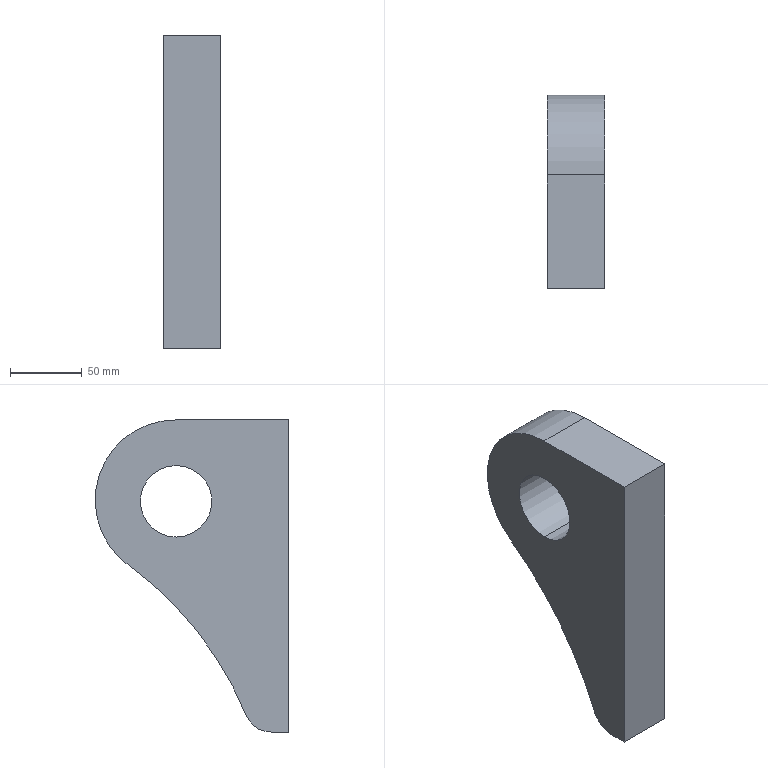Part | SolidWorks | features DeleteBody 1, MBimport 1 | 1 solid | 10 faces | box 40 x 135.266 x 218 mm | volume 706740 mm3 | cylinder 5 | plane 5 | commonest cylinder face diameters 50 x2 38 x1 112 x1 491.554 x1
STEP:
#1=CARTESIAN_POINT('',(-194.,486.644,-1469.814));
#2=VERTEX_POINT('',#1);
#3=CARTESIAN_POINT('',(-194.,486.644,-1419.814));
#4=VERTEX_POINT('',#3);
#5=CARTESIAN_POINT('',(-194.,486.644,-1444.814));
#6=DIRECTION('',(1.,0.,0.));
#7=DIRECTION('',(0.,1.,0.));
#8=AXIS2_PLACEMENT_3D('',#5,#6,#7);
#9=CIRCLE('',#8,25.);
#10=EDGE_CURVE('',#2,#4,#9,.T.);
#11=ORIENTED_EDGE('',*,*,#10,.F.);
#12=CARTESIAN_POINT('',(-154.,486.644,-1469.814));
#13=VERTEX_POINT('',#12);
#14=CARTESIAN_POINT('',(-194.,486.644,-1469.814));
#15=DIRECTION('',(1.,0.,0.));
#16=VECTOR('',#15,1000.);
#17=LINE('',#14,#16);
#18=EDGE_CURVE('',#2,#13,#17,.T.);
#19=ORIENTED_EDGE('',*,*,#18,.T.);
#20=CARTESIAN_POINT('',(-154.,486.644,-1419.814));
#21=VERTEX_POINT('',#20);
#22=CARTESIAN_POINT('',(-154.,486.644,-1444.814));
#23=DIRECTION('',(1.,0.,0.));
#24=DIRECTION('',(0.,1.,0.));
#25=AXIS2_PLACEMENT_3D('',#22,#23,#24);
#26=CIRCLE('',#25,25.);
#27=EDGE_CURVE('',#13,#21,#26,.T.);
#28=ORIENTED_EDGE('',*,*,#27,.T.);
#29=CARTESIAN_POINT('',(-194.,486.644,-1419.814));
#30=DIRECTION('',(1.,0.,0.));
#31=VECTOR('',#30,1000.);
#32=LINE('',#29,#31);
#33=EDGE_CURVE('',#4,#21,#32,.T.);
#34=ORIENTED_EDGE('',*,*,#33,.F.);
#35=EDGE_LOOP('',(#11,#19,#28,#34));
#36=FACE_OUTER_BOUND('',#35,.T.);
#37=CARTESIAN_POINT('',(-194.,486.644,-1444.814));
#38=DIRECTION('',(1.,0.,0.));
#39=DIRECTION('',(0.,0.,1.));
#40=AXIS2_PLACEMENT_3D('',#37,#38,#39);
#41=CYLINDRICAL_SURFACE('',#40,25.);
#42=ADVANCED_FACE('',(#36),#41,.F.);
#43=CARTESIAN_POINT('',(-154.,486.644,-1444.814));
#44=DIRECTION('',(1.,0.,0.));
#45=DIRECTION('',(0.,1.,0.));
#46=AXIS2_PLACEMENT_3D('',#43,#44,#45);
#47=CIRCLE('',#46,25.);
#48=EDGE_CURVE('',#21,#13,#47,.T.);
#49=ORIENTED_EDGE('',*,*,#48,.F.);
#50=ORIENTED_EDGE('',*,*,#27,.F.);
#51=EDGE_LOOP('',(#49,#50));
#52=FACE_BOUND('',#51,.T.);
#53=CARTESIAN_POINT('',(-154.,520.245,-1489.259));
#54=VERTEX_POINT('',#53);
#55=CARTESIAN_POINT('',(-154.,487.266,-1388.));
#56=VERTEX_POINT('',#55);
#57=CARTESIAN_POINT('',(-154.,487.266,-1444.));
#58=DIRECTION('',(1.,0.,0.));
#59=DIRECTION('',(0.,1.,0.));
#60=AXIS2_PLACEMENT_3D('',#57,#58,#59);
#61=CIRCLE('',#60,56.);
#62=EDGE_CURVE('',#54,#56,#61,.T.);
#63=ORIENTED_EDGE('',*,*,#62,.T.);
#64=CARTESIAN_POINT('',(-154.,408.,-1388.));
#65=VERTEX_POINT('',#64);
#66=CARTESIAN_POINT('',(-154.,487.266,-1388.));
#67=DIRECTION('',(0.,-1.,0.));
#68=VECTOR('',#67,1000.);
#69=LINE('',#66,#68);
#70=EDGE_CURVE('',#56,#65,#69,.T.);
#71=ORIENTED_EDGE('',*,*,#70,.T.);
#72=CARTESIAN_POINT('',(-154.,408.,-1606.));
#73=VERTEX_POINT('',#72);
#74=CARTESIAN_POINT('',(-154.,408.,-1388.));
#75=DIRECTION('',(0.,0.,-1.));
#76=VECTOR('',#75,1000.);
#77=LINE('',#74,#76);
#78=EDGE_CURVE('',#65,#73,#77,.T.);
#79=ORIENTED_EDGE('',*,*,#78,.T.);
#80=CARTESIAN_POINT('',(-154.,420.186,-1606.));
#81=VERTEX_POINT('',#80);
#82=CARTESIAN_POINT('',(-154.,408.,-1606.));
#83=DIRECTION('',(0.,1.,0.));
#84=VECTOR('',#83,1000.);
#85=LINE('',#82,#84);
#86=EDGE_CURVE('',#73,#81,#85,.T.);
#87=ORIENTED_EDGE('',*,*,#86,.T.);
#88=CARTESIAN_POINT('',(-154.,437.752,-1594.24));
#89=VERTEX_POINT('',#88);
#90=CARTESIAN_POINT('',(-154.,420.186,-1587.));
#91=DIRECTION('',(1.,0.,0.));
#92=DIRECTION('',(0.,1.,0.));
#93=AXIS2_PLACEMENT_3D('',#90,#91,#92);
#94=CIRCLE('',#93,19.);
#95=EDGE_CURVE('',#81,#89,#94,.T.);
#96=ORIENTED_EDGE('',*,*,#95,.T.);
#97=CARTESIAN_POINT('',(-154.,664.985,-1687.896));
#98=DIRECTION('',(-1.,0.,0.));
#99=DIRECTION('',(0.,1.,0.));
#100=AXIS2_PLACEMENT_3D('',#97,#98,#99);
#101=CIRCLE('',#100,245.777);
#102=EDGE_CURVE('',#89,#54,#101,.T.);
#103=ORIENTED_EDGE('',*,*,#102,.T.);
#104=EDGE_LOOP('',(#63,#71,#79,#87,#96,#103));
#105=FACE_OUTER_BOUND('',#104,.T.);
#106=CARTESIAN_POINT('',(-154.,487.266,-1444.));
#107=DIRECTION('',(1.,0.,0.));
#108=DIRECTION('',(0.,1.,0.));
#109=AXIS2_PLACEMENT_3D('',#106,#107,#108);
#110=PLANE('',#109);
#111=ADVANCED_FACE('',(#52,#105),#110,.T.);
#112=CARTESIAN_POINT('',(-194.,486.644,-1444.814));
#113=DIRECTION('',(1.,0.,0.));
#114=DIRECTION('',(0.,1.,0.));
#115=AXIS2_PLACEMENT_3D('',#112,#113,#114);
#116=CIRCLE('',#115,25.);
#117=EDGE_CURVE('',#4,#2,#116,.T.);
#118=ORIENTED_EDGE('',*,*,#117,.T.);
#119=ORIENTED_EDGE('',*,*,#10,.T.);
#120=EDGE_LOOP('',(#118,#119));
#121=FACE_BOUND('',#120,.T.);
#122=CARTESIAN_POINT('',(-194.,520.245,-1489.259));
#123=VERTEX_POINT('',#122);
#124=CARTESIAN_POINT('',(-194.,487.266,-1388.));
#125=VERTEX_POINT('',#124);
#126=CARTESIAN_POINT('',(-194.,487.266,-1444.));
#127=DIRECTION('',(1.,0.,0.));
#128=DIRECTION('',(0.,1.,0.));
#129=AXIS2_PLACEMENT_3D('',#126,#127,#128);
#130=CIRCLE('',#129,56.);
#131=EDGE_CURVE('',#123,#125,#130,.T.);
#132=ORIENTED_EDGE('',*,*,#131,.F.);
#133=CARTESIAN_POINT('',(-194.,437.752,-1594.24));
#134=VERTEX_POINT('',#133);
#135=CARTESIAN_POINT('',(-194.,664.985,-1687.896));
#136=DIRECTION('',(-1.,0.,0.));
#137=DIRECTION('',(0.,1.,0.));
#138=AXIS2_PLACEMENT_3D('',#135,#136,#137);
#139=CIRCLE('',#138,245.777);
#140=EDGE_CURVE('',#134,#123,#139,.T.);
#141=ORIENTED_EDGE('',*,*,#140,.F.);
#142=CARTESIAN_POINT('',(-194.,420.186,-1606.));
#143=VERTEX_POINT('',#142);
#144=CARTESIAN_POINT('',(-194.,420.186,-1587.));
#145=DIRECTION('',(1.,0.,0.));
#146=DIRECTION('',(0.,1.,0.));
#147=AXIS2_PLACEMENT_3D('',#144,#145,#146);
#148=CIRCLE('',#147,19.);
#149=EDGE_CURVE('',#143,#134,#148,.T.);
#150=ORIENTED_EDGE('',*,*,#149,.F.);
#151=CARTESIAN_POINT('',(-194.,408.,-1606.));
#152=VERTEX_POINT('',#151);
#153=CARTESIAN_POINT('',(-194.,408.,-1606.));
#154=DIRECTION('',(0.,1.,0.));
#155=VECTOR('',#154,1000.);
#156=LINE('',#153,#155);
#157=EDGE_CURVE('',#152,#143,#156,.T.);
#158=ORIENTED_EDGE('',*,*,#157,.F.);
#159=CARTESIAN_POINT('',(-194.,408.,-1388.));
#160=VERTEX_POINT('',#159);
#161=CARTESIAN_POINT('',(-194.,408.,-1388.));
#162=DIRECTION('',(0.,0.,-1.));
#163=VECTOR('',#162,1000.);
#164=LINE('',#161,#163);
#165=EDGE_CURVE('',#160,#152,#164,.T.);
#166=ORIENTED_EDGE('',*,*,#165,.F.);
#167=CARTESIAN_POINT('',(-194.,487.266,-1388.));
#168=DIRECTION('',(0.,-1.,0.));
#169=VECTOR('',#168,1000.);
#170=LINE('',#167,#169);
#171=EDGE_CURVE('',#125,#160,#170,.T.);
#172=ORIENTED_EDGE('',*,*,#171,.F.);
#173=EDGE_LOOP('',(#132,#141,#150,#158,#166,#172));
#174=FACE_OUTER_BOUND('',#173,.T.);
#175=CARTESIAN_POINT('',(-194.,487.266,-1444.));
#176=DIRECTION('',(1.,0.,0.));
#177=DIRECTION('',(0.,1.,0.));
#178=AXIS2_PLACEMENT_3D('',#175,#176,#177);
#179=PLANE('',#178);
#180=ADVANCED_FACE('',(#121,#174),#179,.F.);
#181=ORIENTED_EDGE('',*,*,#18,.F.);
#182=ORIENTED_EDGE('',*,*,#117,.F.);
#183=ORIENTED_EDGE('',*,*,#33,.T.);
#184=ORIENTED_EDGE('',*,*,#48,.T.);
#185=EDGE_LOOP('',(#181,#182,#183,#184));
#186=FACE_OUTER_BOUND('',#185,.T.);
#187=CARTESIAN_POINT('',(-194.,486.644,-1444.814));
#188=DIRECTION('',(1.,0.,0.));
#189=DIRECTION('',(0.,0.,1.));
#190=AXIS2_PLACEMENT_3D('',#187,#188,#189);
#191=CYLINDRICAL_SURFACE('',#190,25.);
#192=ADVANCED_FACE('',(#186),#191,.F.);
#193=ORIENTED_EDGE('',*,*,#102,.F.);
#194=CARTESIAN_POINT('',(-194.,437.752,-1594.24));
#195=DIRECTION('',(1.,0.,0.));
#196=VECTOR('',#195,1000.);
#197=LINE('',#194,#196);
#198=EDGE_CURVE('',#134,#89,#197,.T.);
#199=ORIENTED_EDGE('',*,*,#198,.F.);
#200=ORIENTED_EDGE('',*,*,#140,.T.);
#201=CARTESIAN_POINT('',(-194.,520.245,-1489.259));
#202=DIRECTION('',(1.,0.,0.));
#203=VECTOR('',#202,1000.);
#204=LINE('',#201,#203);
#205=EDGE_CURVE('',#123,#54,#204,.T.);
#206=ORIENTED_EDGE('',*,*,#205,.T.);
#207=EDGE_LOOP('',(#193,#199,#200,#206));
#208=FACE_OUTER_BOUND('',#207,.T.);
#209=CARTESIAN_POINT('',(-194.,664.985,-1687.896));
#210=DIRECTION('',(1.,0.,0.));
#211=DIRECTION('',(0.,0.,1.));
#212=AXIS2_PLACEMENT_3D('',#209,#210,#211);
#213=CYLINDRICAL_SURFACE('',#212,245.777);
#214=ADVANCED_FACE('',(#208),#213,.F.);
#215=ORIENTED_EDGE('',*,*,#95,.F.);
#216=CARTESIAN_POINT('',(-194.,420.186,-1606.));
#217=DIRECTION('',(1.,0.,0.));
#218=VECTOR('',#217,1000.);
#219=LINE('',#216,#218);
#220=EDGE_CURVE('',#143,#81,#219,.T.);
#221=ORIENTED_EDGE('',*,*,#220,.F.);
#222=ORIENTED_EDGE('',*,*,#149,.T.);
#223=ORIENTED_EDGE('',*,*,#198,.T.);
#224=EDGE_LOOP('',(#215,#221,#222,#223));
#225=FACE_OUTER_BOUND('',#224,.T.);
#226=CARTESIAN_POINT('',(-194.,420.186,-1587.));
#227=DIRECTION('',(1.,0.,0.));
#228=DIRECTION('',(0.,0.,1.));
#229=AXIS2_PLACEMENT_3D('',#226,#227,#228);
#230=CYLINDRICAL_SURFACE('',#229,19.);
#231=ADVANCED_FACE('',(#225),#230,.T.);
#232=ORIENTED_EDGE('',*,*,#86,.F.);
#233=CARTESIAN_POINT('',(-194.,408.,-1606.));
#234=DIRECTION('',(1.,0.,0.));
#235=VECTOR('',#234,1000.);
#236=LINE('',#233,#235);
#237=EDGE_CURVE('',#152,#73,#236,.T.);
#238=ORIENTED_EDGE('',*,*,#237,.F.);
#239=ORIENTED_EDGE('',*,*,#157,.T.);
#240=ORIENTED_EDGE('',*,*,#220,.T.);
#241=EDGE_LOOP('',(#232,#238,#239,#240));
#242=FACE_OUTER_BOUND('',#241,.T.);
#243=CARTESIAN_POINT('',(-194.,408.,-1606.));
#244=DIRECTION('',(0.,0.,-1.));
#245=DIRECTION('',(0.,-1.,0.));
#246=AXIS2_PLACEMENT_3D('',#243,#244,#245);
#247=PLANE('',#246);
#248=ADVANCED_FACE('',(#242),#247,.T.);
#249=ORIENTED_EDGE('',*,*,#78,.F.);
#250=CARTESIAN_POINT('',(-194.,408.,-1388.));
#251=DIRECTION('',(1.,0.,0.));
#252=VECTOR('',#251,1000.);
#253=LINE('',#250,#252);
#254=EDGE_CURVE('',#160,#65,#253,.T.);
#255=ORIENTED_EDGE('',*,*,#254,.F.);
#256=ORIENTED_EDGE('',*,*,#165,.T.);
#257=ORIENTED_EDGE('',*,*,#237,.T.);
#258=EDGE_LOOP('',(#249,#255,#256,#257));
#259=FACE_OUTER_BOUND('',#258,.T.);
#260=CARTESIAN_POINT('',(-194.,408.,-1388.));
#261=DIRECTION('',(0.,-1.,0.));
#262=DIRECTION('',(0.,0.,-1.));
#263=AXIS2_PLACEMENT_3D('',#260,#261,#262);
#264=PLANE('',#263);
#265=ADVANCED_FACE('',(#259),#264,.T.);
#266=ORIENTED_EDGE('',*,*,#70,.F.);
#267=CARTESIAN_POINT('',(-194.,487.266,-1388.));
#268=DIRECTION('',(1.,0.,0.));
#269=VECTOR('',#268,1000.);
#270=LINE('',#267,#269);
#271=EDGE_CURVE('',#125,#56,#270,.T.);
#272=ORIENTED_EDGE('',*,*,#271,.F.);
#273=ORIENTED_EDGE('',*,*,#171,.T.);
#274=ORIENTED_EDGE('',*,*,#254,.T.);
#275=EDGE_LOOP('',(#266,#272,#273,#274));
#276=FACE_OUTER_BOUND('',#275,.T.);
#277=CARTESIAN_POINT('',(-194.,487.266,-1388.));
#278=DIRECTION('',(0.,0.,1.));
#279=DIRECTION('',(1.,0.,0.));
#280=AXIS2_PLACEMENT_3D('',#277,#278,#279);
#281=PLANE('',#280);
#282=ADVANCED_FACE('',(#276),#281,.T.);
#283=ORIENTED_EDGE('',*,*,#62,.F.);
#284=ORIENTED_EDGE('',*,*,#205,.F.);
#285=ORIENTED_EDGE('',*,*,#131,.T.);
#286=ORIENTED_EDGE('',*,*,#271,.T.);
#287=EDGE_LOOP('',(#283,#284,#285,#286));
#288=FACE_OUTER_BOUND('',#287,.T.);
#289=CARTESIAN_POINT('',(-194.,487.266,-1444.));
#290=DIRECTION('',(1.,0.,0.));
#291=DIRECTION('',(0.,0.,1.));
#292=AXIS2_PLACEMENT_3D('',#289,#290,#291);
#293=CYLINDRICAL_SURFACE('',#292,56.);
#294=ADVANCED_FACE('',(#288),#293,.T.);
#295=CLOSED_SHELL('',(#42,#111,#180,#192,#214,#231,#248,#265,#282,#294));
#296=MANIFOLD_SOLID_BREP('',#295);
#297=CARTESIAN_POINT('',(0.,0.,0.));
#298=DIRECTION('',(0.,0.,1.));
#299=DIRECTION('',(1.,0.,0.));
#300=AXIS2_PLACEMENT_3D('',#297,#298,#299);
#301=(LENGTH_UNIT()NAMED_UNIT(*)SI_UNIT(.MILLI.,.METRE.));
#302=UNCERTAINTY_MEASURE_WITH_UNIT(LENGTH_MEASURE(0.00001),#301,'','');
#303=(NAMED_UNIT(*)PLANE_ANGLE_UNIT()SI_UNIT($,.RADIAN.));
#304=(NAMED_UNIT(*)SI_UNIT($,.STERADIAN.)SOLID_ANGLE_UNIT());
#305=(GEOMETRIC_REPRESENTATION_CONTEXT(3)GLOBAL_UNCERTAINTY_ASSIGNED_CONTEXT((#302))GLOBAL_UNIT_ASSIGNED_CONTEXT((#301,#303,#304))REPRESENTATION_CONTEXT('',''));
#306=ADVANCED_BREP_SHAPE_REPRESENTATION('',(#296,#300),#305);